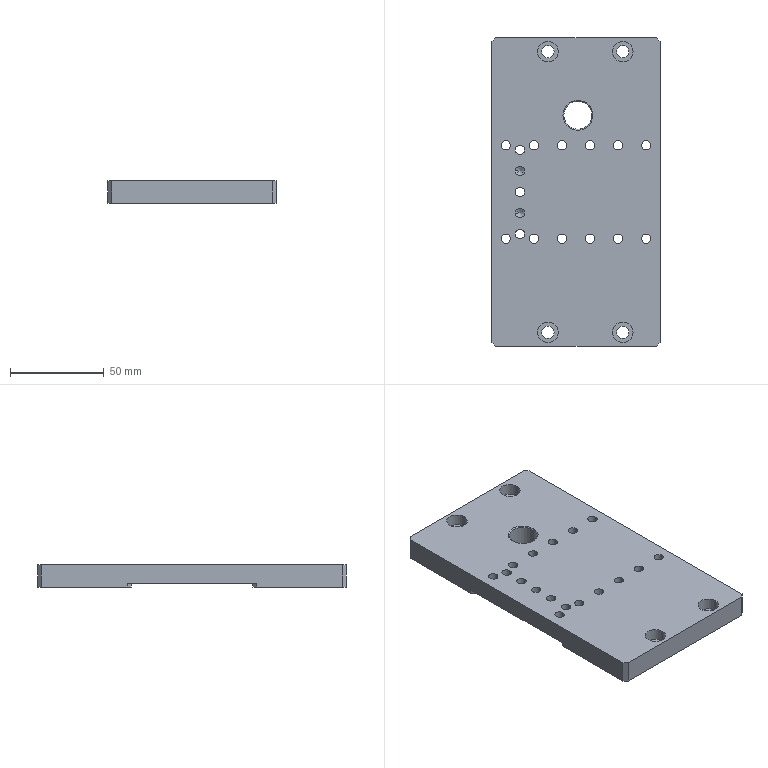NC program | NX | posted with a generic post | part box 90 x 165 x 12 mm
Whole program:
N10 G17 G21 G94 G90
(FLOOR_WALL_1 , TOOL : D10)
N12 T15 M6
N14 G54
N16 G17 G0 G90 X81.057 Y96.5 S9500 M3
N18 G43 Z30. H15
N20 Z0.55
N22 G94 G1 Z-0.95 F1000.
N24 X81.634 Y95.5
N26 G3 X82.5 Y95. R1.
N28 G1 X114.788 F3500.
N30 X109.94 Y90.152
N32 Y-0.152
N34 X114.758 Y-4.97
N36 X50.242
N38 X55.06 Y-0.152
N40 Y90.152
N42 X50.212 Y95.
N44 X82.5
N46 Y90.
N48 X104.94
N50 Y0.
N52 X60.06
N54 Y90.
N56 X82.5
N58 Y85.
N60 X99.94
N62 Y5.
N64 X65.06
N66 Y85.
N68 X82.5
N70 Y80.
N72 X94.94
N74 Y10.
N76 X70.06
N78 Y80.
N80 X82.5
N82 Y75.
N84 X89.94
N86 Y15.
N88 X75.06
N90 Y75.
N92 X82.5
N94 Y70.
N96 X84.94
N98 Y20.
N100 X80.06
N102 Y70.
N104 X82.5
N106 G3 X83.366 Y70.5 R1.
N108 G1 Z0.55
N110 G0 X81.057 Y96.5 Z-0.4
N112 G1 Z-1.9 F1000.
N114 X81.634 Y95.5
N116 G3 X82.5 Y95. R1.
N118 G1 X114.788 F3500.
N120 X109.94 Y90.152
N122 Y-0.152
N124 X114.758 Y-4.97
N126 X50.242
N128 X55.06 Y-0.152
N130 Y90.152
N132 X50.212 Y95.
N134 X82.5
N136 Y90.
N138 X104.94
N140 Y0.
N142 X60.06
N144 Y90.
N146 X82.5
N148 Y85.
N150 X99.94
N152 Y5.
N154 X65.06
N156 Y85.
N158 X82.5
N160 Y80.
N162 X94.94
N164 Y10.
N166 X70.06
N168 Y80.
N170 X82.5
N172 Y75.
N174 X89.94
N176 Y15.
N178 X75.06
N180 Y75.
N182 X82.5
N184 Y70.
N186 X84.94
N188 Y20.
N190 X80.06
N192 Y70.
N194 X82.5
N196 G3 X83.366 Y70.5 R1.
N198 G1 Z-0.4
N200 G0 Z30.
N202 M5
(FLOOR_WALL_1_COPY , TOOL : D10JING)
N204 T14 M6
N206 G54
N208 G17 G0 G90 X111.137 Y96.5 S9500 M3
N210 G43 Z30. H14
N212 Z-0.5
N214 G94 G1 Z-2. F1000.
N216 X110.039 Y95.866
N218 G3 X109.539 Y95. R1.
N220 G1 Y-5. F1500.
N222 X104.623
N224 Y95.
N226 X99.706
N228 Y-5.
N230 X94.79
N232 Y95.
N234 X89.874
N236 Y-5.
N238 X84.958
N240 Y95.
N242 X80.041
N244 Y-5.
N246 X75.125
N248 Y95.
N250 X70.209
N252 Y-5.
N254 X65.293
N256 Y95.
N258 X60.376
N260 Y-5.
N262 X55.46
N264 Y95.
N266 G2 X55.96 Y95.866 R1.
N268 G1 X57.058 Y96.5
N270 Z-0.5
N272 G0 X49.955
N274 G1 Z-2. F1000.
N276 X49.812 Y95.966
N278 G3 X50.071 Y95. R1.
N280 G1 X54.96 Y90.111 F1500.
N282 Y-0.111
N284 X50.081 Y-4.99
N286 G3 X49.822 Y-5.956 R1.
N288 G1 X49.968 Y-6.5
N290 Z-0.5
N292 G0 X115.045
N294 G1 Z-2. F1000.
N296 X115.188 Y-5.966
N298 G3 X114.929 Y-5. R1.
N300 G1 X110.04 Y-0.111 F1500.
N302 Y90.111
N304 X114.929 Y95.
N306 G3 X115.188 Y95.966 R1.
N308 G1 X115.045 Y96.5
N310 Z-0.5
N312 G0 Z30.
N314 M5
(PLANAR_MILL_COPY_COPY_1 , TOOL : D6A45)
N316 T01 M6
N318 G54
N320 G17 G0 G90 X5.6 Y70.866 S9500 M3
N322 G43 Z30. H1
N324 Z0.5
N326 G94 G1 Z-1. F1250.
N328 G3 X5.1 Y70. R1.
N330 X7.5 Y67.6 R2.4
N332 X5.1 Y70. R-2.4
N334 X5.6 Y69.134 R1.
N336 G1 Z0.5
N338 G0 Z30.
N340 Y30.866
N342 Z0.5
N344 G1 Z-1.
N346 G3 X5.1 Y30. R1.
N348 X7.5 Y27.6 R2.4
N350 X5.1 Y30. R-2.4
N352 X5.6 Y29.134 R1.
N354 G1 Z0.5
N356 G0 Z30.
N358 X-1.4 Y44.134
N360 Z0.5
N362 G1 Z-1.
N364 G3 X-0.9 Y45. R1.
N366 G1 Y88.
N368 G2 X-0.636 Y88.636 R0.9
N370 G1 X1.364 Y90.636
N372 G2 X2. Y90.9 R0.9
N374 G1 X48.
N376 G2 X48.636 Y90.636 R0.9
N378 G1 X50.596 Y88.676
N380 G2 X50.86 Y88.04 R0.9
N382 G1 Y1.96
N384 G2 X50.596 Y1.324 R0.9
N386 G1 X48.636 Y-0.636
N388 G2 X48. Y-0.9 R0.9
N390 G1 X2.
N392 G2 X1.364 Y-0.636 R0.9
N394 G1 X-0.636 Y1.364
N396 G2 X-0.9 Y2. R0.9
N398 G1 Y45.
N400 G3 X-1.4 Y45.866 R1.
N402 G1 Z0.5
N404 G0 Z30.
N406 X166.4
N408 Z0.5
N410 G1 Z-1.
N412 G3 X165.9 Y45. R1.
N414 G1 Y2.
N416 G2 X165.636 Y1.364 R0.9
N418 G1 X163.636 Y-0.636
N420 G2 X163. Y-0.9 R0.9
N422 G1 X117.
N424 G2 X116.364 Y-0.636 R0.9
N426 G1 X114.404 Y1.324
N428 G2 X114.14 Y1.96 R0.9
N430 G1 Y88.04
N432 G2 X114.404 Y88.676 R0.9
N434 G1 X116.364 Y90.636
N436 G2 X117. Y90.9 R0.9
N438 G1 X163.
N440 G2 X163.636 Y90.636 R0.9
N442 G1 X165.636 Y88.636
N444 G2 X165.9 Y88. R0.9
N446 G1 Y45.
N448 G3 X166.4 Y44.134 R1.
N450 G1 Z0.5
N452 G0 Z30.
N454 X159.4 Y29.134
N456 Z0.5
N458 G1 Z-1.
N460 G3 X159.9 Y30. R1.
N462 X157.5 Y32.4 R2.4
N464 X159.9 Y30. R-2.4
N466 X159.4 Y30.866 R1.
N468 G1 Z0.5
N470 G0 Z30.
N472 Y69.134
N474 Z0.5
N476 G1 Z-1.
N478 G3 X159.9 Y70. R1.
N480 X157.5 Y72.4 R2.4
N482 X159.9 Y70. R-2.4
N484 X159.4 Y70.866 R1.
N486 G1 Z0.5
N488 G0 Z30.
(PLANAR_MILL_COPY_COPY_COPY , TOOL : D6A45)
N490 X122.634 Y40.
N492 Z0.
N494 G1 Z-1.5
N496 G3 X123.5 Y39.5 R1.
N498 X130. Y46. R6.5
N500 X123.5 Y39.5 R-6.5
N502 X124.366 Y40. R1.
N504 G1 Z0.
N506 G0 Z30.
(PLANAR_MILL_COPY_COPY_1_COPY , TOOL : D6A45)
N508 X57.747 Y82.814
N510 Z-1.5
N512 G1 Z-3.
N514 X58.366 Y83.6
N516 G3 X57.5 Y84.1 R1.
N518 X55.9 Y82.5 R1.6
N520 X57.5 Y84.1 R-1.6
N522 X56.634 Y83.6 R1.
N524 G1 X57.253 Y82.814
N526 Z-1.5
N528 G0 Z30.
N530 X57.747 Y67.814
N532 Z-1.5
N534 G1 Z-3.
N536 X58.366 Y68.6
N538 G3 X57.5 Y69.1 R1.
N540 X55.9 Y67.5 R1.6
N542 X57.5 Y69.1 R-1.6
N544 X56.634 Y68.6 R1.
N546 G1 X57.253 Y67.814
N548 Z-1.5
N550 G0 Z30.
N552 X57.747 Y52.814
N554 Z-1.5
N556 G1 Z-3.
N558 X58.366 Y53.6
N560 G3 X57.5 Y54.1 R1.
N562 X55.9 Y52.5 R1.6
N564 X57.5 Y54.1 R-1.6
N566 X56.634 Y53.6 R1.
N568 G1 X57.253 Y52.814
N570 Z-1.5
N572 G0 Z30.
N574 Y37.186
N576 Z-1.5
N578 G1 Z-3.
N580 X56.634 Y36.4
N582 G3 X57.5 Y35.9 R1.
N584 X59.1 Y37.5 R1.6
N586 X57.5 Y35.9 R-1.6
N588 X58.366 Y36.4 R1.
N590 G1 X57.747 Y37.186
N592 Z-1.5
N594 G0 Z30.
N596 X57.253 Y22.186
N598 Z-1.5
N600 G1 Z-3.
N602 X56.634 Y21.4
N604 G3 X57.5 Y20.9 R1.
N606 X59.1 Y22.5 R1.6
N608 X57.5 Y20.9 R-1.6
N610 X58.366 Y21.4 R1.
N612 G1 X57.747 Y22.186
N614 Z-1.5
N616 G0 Z30.
N618 X57.253 Y7.186
N620 Z-1.5
N622 G1 Z-3.
N624 X56.634 Y6.4
N626 G3 X57.5 Y5.9 R1.
N628 X59.1 Y7.5 R1.6
N630 X57.5 Y5.9 R-1.6
N632 X58.366 Y6.4 R1.
N634 G1 X57.747 Y7.186
N636 Z-1.5
N638 G0 Z30.
N640 X59.753 Y14.686
N642 Z-1.5
N644 G1 Z-3.
N646 X59.134 Y13.9
N648 G3 X60. Y13.4 R1.
N650 X61.6 Y15. R1.6
N652 X60. Y13.4 R-1.6
N654 X60.866 Y13.9 R1.
N656 G1 X60.247 Y14.686
N658 Z-1.5
N660 G0 Z30.
N662 X82.253
N664 Z-1.5
N666 G1 Z-3.
N668 X81.634 Y13.9
N670 G3 X82.5 Y13.4 R1.
N672 X84.1 Y15. R1.6
N674 X82.5 Y13.4 R-1.6
N676 X83.366 Y13.9 R1.
N678 G1 X82.747 Y14.686
N680 Z-1.5
N682 G0 Z30.
N684 X113. Y-2.647
N686 Z-1.5
N688 G1 Z-3.
N690 X113.209 Y-1.866
N692 G3 X112.95 Y-0.9 R1.
N694 G1 X52.05
N696 G3 X51.791 Y-1.866 R1.
N698 G1 X52. Y-2.647
N700 Z-1.5
N702 G0 Z30.
N704 Y92.647
N706 Z-1.5
N708 G1 Z-3.
N710 X51.791 Y91.866
N712 G3 X52.05 Y90.9 R1.
N714 G1 X112.95
N716 G3 X113.209 Y91.866 R1.
N718 G1 X113. Y92.647
N720 Z-1.5
N722 G0 Z30.
N724 X104.753 Y14.686
N726 Z-1.5
N728 G1 Z-3.
N730 X104.134 Y13.9
N732 G3 X105. Y13.4 R1.
N734 X106.6 Y15. R1.6
N736 X105. Y13.4 R-1.6
N738 X105.866 Y13.9 R1.
N740 G1 X105.247 Y14.686
N742 Z-1.5
N744 G0 Z30.
N746 X107.253 Y7.186
N748 Z-1.5
N750 G1 Z-3.
N752 X106.634 Y6.4
N754 G3 X107.5 Y5.9 R1.
N756 X109.1 Y7.5 R1.6
N758 X107.5 Y5.9 R-1.6
N760 X108.366 Y6.4 R1.
N762 G1 X107.747 Y7.186
N764 Z-1.5
N766 G0 Z30.
N768 X107.253 Y22.186
N770 Z-1.5
N772 G1 Z-3.
N774 X106.634 Y21.4
N776 G3 X107.5 Y20.9 R1.
N778 X109.1 Y22.5 R1.6
N780 X107.5 Y20.9 R-1.6
N782 X108.366 Y21.4 R1.
N784 G1 X107.747 Y22.186
N786 Z-1.5
N788 G0 Z30.
N790 X107.253 Y37.186
N792 Z-1.5
N794 G1 Z-3.
N796 X106.634 Y36.4
N798 G3 X107.5 Y35.9 R1.
N800 X109.1 Y37.5 R1.6
N802 X107.5 Y35.9 R-1.6
N804 X108.366 Y36.4 R1.
N806 G1 X107.747 Y37.186
N808 Z-1.5
N810 G0 Z30.
N812 Y52.814
N814 Z-1.5
N816 G1 Z-3.
N818 X108.366 Y53.6
N820 G3 X107.5 Y54.1 R1.
N822 X105.9 Y52.5 R1.6
N824 X107.5 Y54.1 R-1.6
N826 X106.634 Y53.6 R1.
N828 G1 X107.253 Y52.814
N830 Z-1.5
N832 G0 Z30.
N834 X107.747 Y67.814
N836 Z-1.5
N838 G1 Z-3.
N840 X108.366 Y68.6
N842 G3 X107.5 Y69.1 R1.
N844 X105.9 Y67.5 R1.6
N846 X107.5 Y69.1 R-1.6
N848 X106.634 Y68.6 R1.
N850 G1 X107.253 Y67.814
N852 Z-1.5
N854 G0 Z30.
N856 X107.747 Y82.814
N858 Z-1.5
N860 G1 Z-3.
N862 X108.366 Y83.6
N864 G3 X107.5 Y84.1 R1.
N866 X105.9 Y82.5 R1.6
N868 X107.5 Y84.1 R-1.6
N870 X106.634 Y83.6 R1.
N872 G1 X107.253 Y82.814
N874 Z-1.5
N876 G0 Z30.
N878 M5
N880 M2